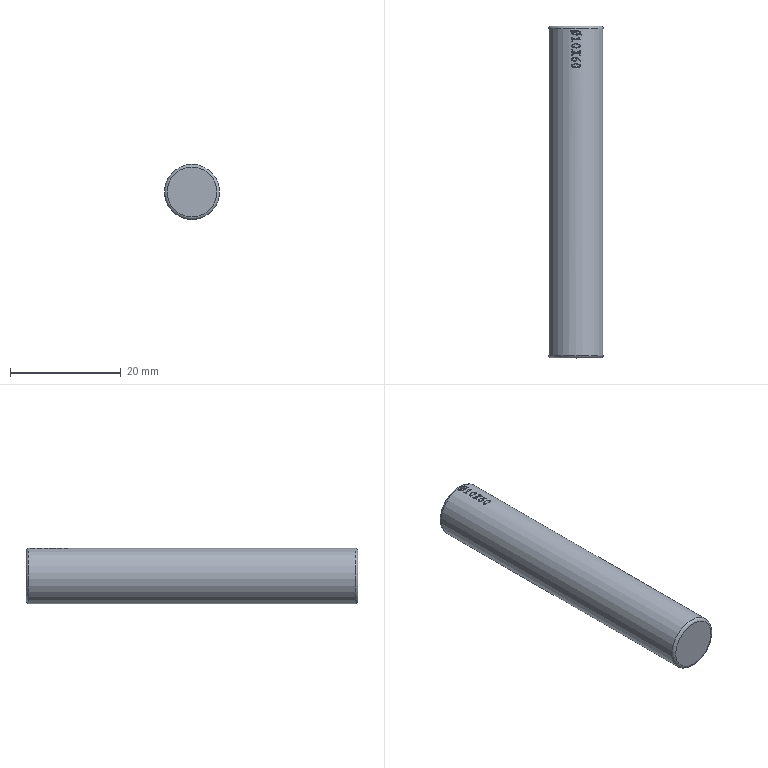Part | STEP file | solid 56 | 1 solid | 77 faces | box 10 x 60 x 10 mm | volume 4502 mm3 | plane 38 | other 29 | cylinder 7 | torus 2 | cone 1 | commonest cylinder face diameters 10 x6 5 x1